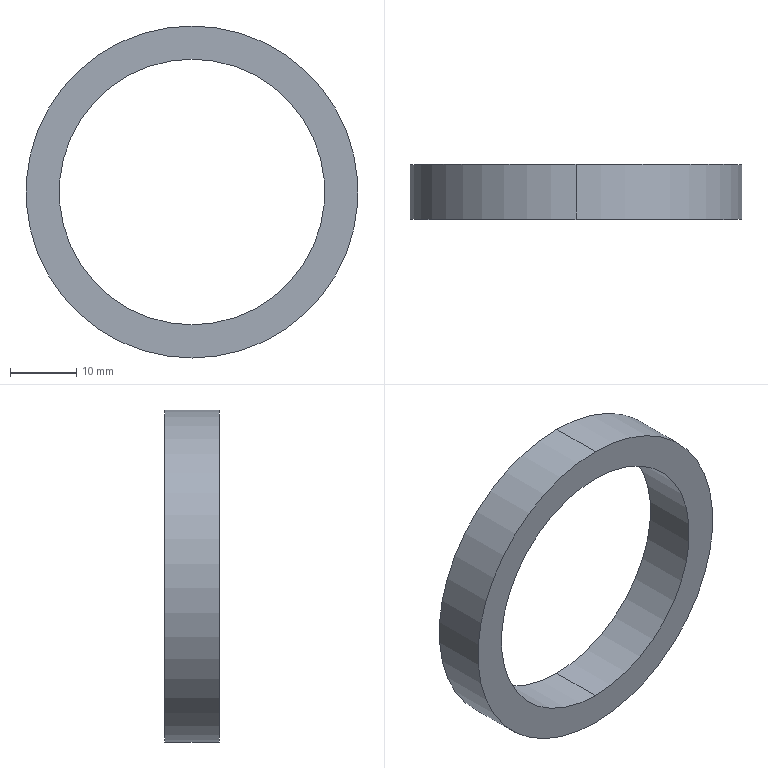Part | STEP file | Produce dryer shaft collar | 1 solid | 6 faces | box 50 x 8.25 x 50 mm | volume 5832 mm3 | cylinder 4 | plane 2 | commonest cylinder face diameters 40 x2 50 x2
STEP:
#1=CARTESIAN_POINT('',(0.,8.25,-20.));
#2=VERTEX_POINT('',#1);
#3=CARTESIAN_POINT('',(0.,8.25,20.));
#4=VERTEX_POINT('',#3);
#5=CARTESIAN_POINT('',(0.,8.25,0.));
#6=DIRECTION('',(0.,1.,0.));
#7=DIRECTION('',(0.,0.,1.));
#8=AXIS2_PLACEMENT_3D('',#5,#6,#7);
#9=CIRCLE('',#8,20.);
#10=EDGE_CURVE('',#2,#4,#9,.T.);
#11=ORIENTED_EDGE('',*,*,#10,.T.);
#12=CARTESIAN_POINT('',(0.,0.,20.));
#13=VERTEX_POINT('',#12);
#14=CARTESIAN_POINT('',(0.,8.25,20.));
#15=DIRECTION('',(0.,-1.,0.));
#16=VECTOR('',#15,1000.);
#17=LINE('',#14,#16);
#18=EDGE_CURVE('',#4,#13,#17,.T.);
#19=ORIENTED_EDGE('',*,*,#18,.T.);
#20=CARTESIAN_POINT('',(0.,0.,-20.));
#21=VERTEX_POINT('',#20);
#22=CARTESIAN_POINT('',(0.,0.,0.));
#23=DIRECTION('',(0.,1.,0.));
#24=DIRECTION('',(0.,0.,1.));
#25=AXIS2_PLACEMENT_3D('',#22,#23,#24);
#26=CIRCLE('',#25,20.);
#27=EDGE_CURVE('',#21,#13,#26,.T.);
#28=ORIENTED_EDGE('',*,*,#27,.F.);
#29=CARTESIAN_POINT('',(0.,8.25,-20.));
#30=DIRECTION('',(0.,-1.,0.));
#31=VECTOR('',#30,1000.);
#32=LINE('',#29,#31);
#33=EDGE_CURVE('',#2,#21,#32,.T.);
#34=ORIENTED_EDGE('',*,*,#33,.F.);
#35=EDGE_LOOP('',(#11,#19,#28,#34));
#36=FACE_OUTER_BOUND('',#35,.T.);
#37=CARTESIAN_POINT('',(0.,8.25,0.));
#38=DIRECTION('',(0.,-1.,0.));
#39=DIRECTION('',(0.,0.,-1.));
#40=AXIS2_PLACEMENT_3D('',#37,#38,#39);
#41=CYLINDRICAL_SURFACE('',#40,20.);
#42=ADVANCED_FACE('',(#36),#41,.F.);
#43=CARTESIAN_POINT('',(0.,8.25,25.));
#44=VERTEX_POINT('',#43);
#45=CARTESIAN_POINT('',(0.,8.25,-25.));
#46=VERTEX_POINT('',#45);
#47=CARTESIAN_POINT('',(0.,8.25,0.));
#48=DIRECTION('',(0.,1.,0.));
#49=DIRECTION('',(0.,0.,1.));
#50=AXIS2_PLACEMENT_3D('',#47,#48,#49);
#51=CIRCLE('',#50,25.);
#52=EDGE_CURVE('',#44,#46,#51,.T.);
#53=ORIENTED_EDGE('',*,*,#52,.F.);
#54=CARTESIAN_POINT('',(0.,0.,25.));
#55=VERTEX_POINT('',#54);
#56=CARTESIAN_POINT('',(0.,8.25,25.));
#57=DIRECTION('',(0.,-1.,0.));
#58=VECTOR('',#57,1000.);
#59=LINE('',#56,#58);
#60=EDGE_CURVE('',#44,#55,#59,.T.);
#61=ORIENTED_EDGE('',*,*,#60,.T.);
#62=CARTESIAN_POINT('',(0.,0.,-25.));
#63=VERTEX_POINT('',#62);
#64=CARTESIAN_POINT('',(0.,0.,0.));
#65=DIRECTION('',(0.,1.,0.));
#66=DIRECTION('',(0.,0.,1.));
#67=AXIS2_PLACEMENT_3D('',#64,#65,#66);
#68=CIRCLE('',#67,25.);
#69=EDGE_CURVE('',#55,#63,#68,.T.);
#70=ORIENTED_EDGE('',*,*,#69,.T.);
#71=CARTESIAN_POINT('',(0.,8.25,-25.));
#72=DIRECTION('',(0.,-1.,0.));
#73=VECTOR('',#72,1000.);
#74=LINE('',#71,#73);
#75=EDGE_CURVE('',#46,#63,#74,.T.);
#76=ORIENTED_EDGE('',*,*,#75,.F.);
#77=EDGE_LOOP('',(#53,#61,#70,#76));
#78=FACE_OUTER_BOUND('',#77,.T.);
#79=CARTESIAN_POINT('',(0.,8.25,0.));
#80=DIRECTION('',(0.,-1.,0.));
#81=DIRECTION('',(0.,0.,-1.));
#82=AXIS2_PLACEMENT_3D('',#79,#80,#81);
#83=CYLINDRICAL_SURFACE('',#82,25.);
#84=ADVANCED_FACE('',(#78),#83,.T.);
#85=CARTESIAN_POINT('',(0.,8.25,0.));
#86=DIRECTION('',(0.,1.,0.));
#87=DIRECTION('',(0.,0.,1.));
#88=AXIS2_PLACEMENT_3D('',#85,#86,#87);
#89=CIRCLE('',#88,25.);
#90=EDGE_CURVE('',#46,#44,#89,.T.);
#91=ORIENTED_EDGE('',*,*,#90,.T.);
#92=ORIENTED_EDGE('',*,*,#52,.T.);
#93=EDGE_LOOP('',(#91,#92));
#94=FACE_OUTER_BOUND('',#93,.T.);
#95=ORIENTED_EDGE('',*,*,#10,.F.);
#96=CARTESIAN_POINT('',(0.,8.25,0.));
#97=DIRECTION('',(0.,1.,0.));
#98=DIRECTION('',(0.,0.,1.));
#99=AXIS2_PLACEMENT_3D('',#96,#97,#98);
#100=CIRCLE('',#99,20.);
#101=EDGE_CURVE('',#4,#2,#100,.T.);
#102=ORIENTED_EDGE('',*,*,#101,.F.);
#103=EDGE_LOOP('',(#95,#102));
#104=FACE_BOUND('',#103,.T.);
#105=CARTESIAN_POINT('',(0.,8.25,0.));
#106=DIRECTION('',(0.,1.,0.));
#107=DIRECTION('',(0.,0.,1.));
#108=AXIS2_PLACEMENT_3D('',#105,#106,#107);
#109=PLANE('',#108);
#110=ADVANCED_FACE('',(#94,#104),#109,.T.);
#111=CARTESIAN_POINT('',(0.,0.,0.));
#112=DIRECTION('',(0.,1.,0.));
#113=DIRECTION('',(0.,0.,1.));
#114=AXIS2_PLACEMENT_3D('',#111,#112,#113);
#115=CIRCLE('',#114,25.);
#116=EDGE_CURVE('',#63,#55,#115,.T.);
#117=ORIENTED_EDGE('',*,*,#116,.F.);
#118=ORIENTED_EDGE('',*,*,#69,.F.);
#119=EDGE_LOOP('',(#117,#118));
#120=FACE_OUTER_BOUND('',#119,.T.);
#121=ORIENTED_EDGE('',*,*,#27,.T.);
#122=CARTESIAN_POINT('',(0.,0.,0.));
#123=DIRECTION('',(0.,1.,0.));
#124=DIRECTION('',(0.,0.,1.));
#125=AXIS2_PLACEMENT_3D('',#122,#123,#124);
#126=CIRCLE('',#125,20.);
#127=EDGE_CURVE('',#13,#21,#126,.T.);
#128=ORIENTED_EDGE('',*,*,#127,.T.);
#129=EDGE_LOOP('',(#121,#128));
#130=FACE_BOUND('',#129,.T.);
#131=CARTESIAN_POINT('',(0.,0.,0.));
#132=DIRECTION('',(0.,1.,0.));
#133=DIRECTION('',(0.,0.,1.));
#134=AXIS2_PLACEMENT_3D('',#131,#132,#133);
#135=PLANE('',#134);
#136=ADVANCED_FACE('',(#120,#130),#135,.F.);
#137=ORIENTED_EDGE('',*,*,#60,.F.);
#138=ORIENTED_EDGE('',*,*,#90,.F.);
#139=ORIENTED_EDGE('',*,*,#75,.T.);
#140=ORIENTED_EDGE('',*,*,#116,.T.);
#141=EDGE_LOOP('',(#137,#138,#139,#140));
#142=FACE_OUTER_BOUND('',#141,.T.);
#143=CARTESIAN_POINT('',(0.,8.25,0.));
#144=DIRECTION('',(0.,-1.,0.));
#145=DIRECTION('',(0.,0.,-1.));
#146=AXIS2_PLACEMENT_3D('',#143,#144,#145);
#147=CYLINDRICAL_SURFACE('',#146,25.);
#148=ADVANCED_FACE('',(#142),#147,.T.);
#149=ORIENTED_EDGE('',*,*,#18,.F.);
#150=ORIENTED_EDGE('',*,*,#101,.T.);
#151=ORIENTED_EDGE('',*,*,#33,.T.);
#152=ORIENTED_EDGE('',*,*,#127,.F.);
#153=EDGE_LOOP('',(#149,#150,#151,#152));
#154=FACE_OUTER_BOUND('',#153,.T.);
#155=CARTESIAN_POINT('',(0.,8.25,0.));
#156=DIRECTION('',(0.,-1.,0.));
#157=DIRECTION('',(0.,0.,-1.));
#158=AXIS2_PLACEMENT_3D('',#155,#156,#157);
#159=CYLINDRICAL_SURFACE('',#158,20.);
#160=ADVANCED_FACE('',(#154),#159,.F.);
#161=CLOSED_SHELL('',(#42,#84,#110,#136,#148,#160));
#162=MANIFOLD_SOLID_BREP('',#161);
#163=CARTESIAN_POINT('',(0.,0.,0.));
#164=DIRECTION('',(0.,0.,1.));
#165=DIRECTION('',(1.,0.,0.));
#166=AXIS2_PLACEMENT_3D('',#163,#164,#165);
#167=(LENGTH_UNIT()NAMED_UNIT(*)SI_UNIT(.MILLI.,.METRE.));
#168=UNCERTAINTY_MEASURE_WITH_UNIT(LENGTH_MEASURE(0.00001),#167,'','');
#169=(NAMED_UNIT(*)PLANE_ANGLE_UNIT()SI_UNIT($,.RADIAN.));
#170=(NAMED_UNIT(*)SI_UNIT($,.STERADIAN.)SOLID_ANGLE_UNIT());
#171=(GEOMETRIC_REPRESENTATION_CONTEXT(3)GLOBAL_UNCERTAINTY_ASSIGNED_CONTEXT((#168))GLOBAL_UNIT_ASSIGNED_CONTEXT((#167,#169,#170))REPRESENTATION_CONTEXT('',''));
#172=ADVANCED_BREP_SHAPE_REPRESENTATION('',(#162,#166),#171);